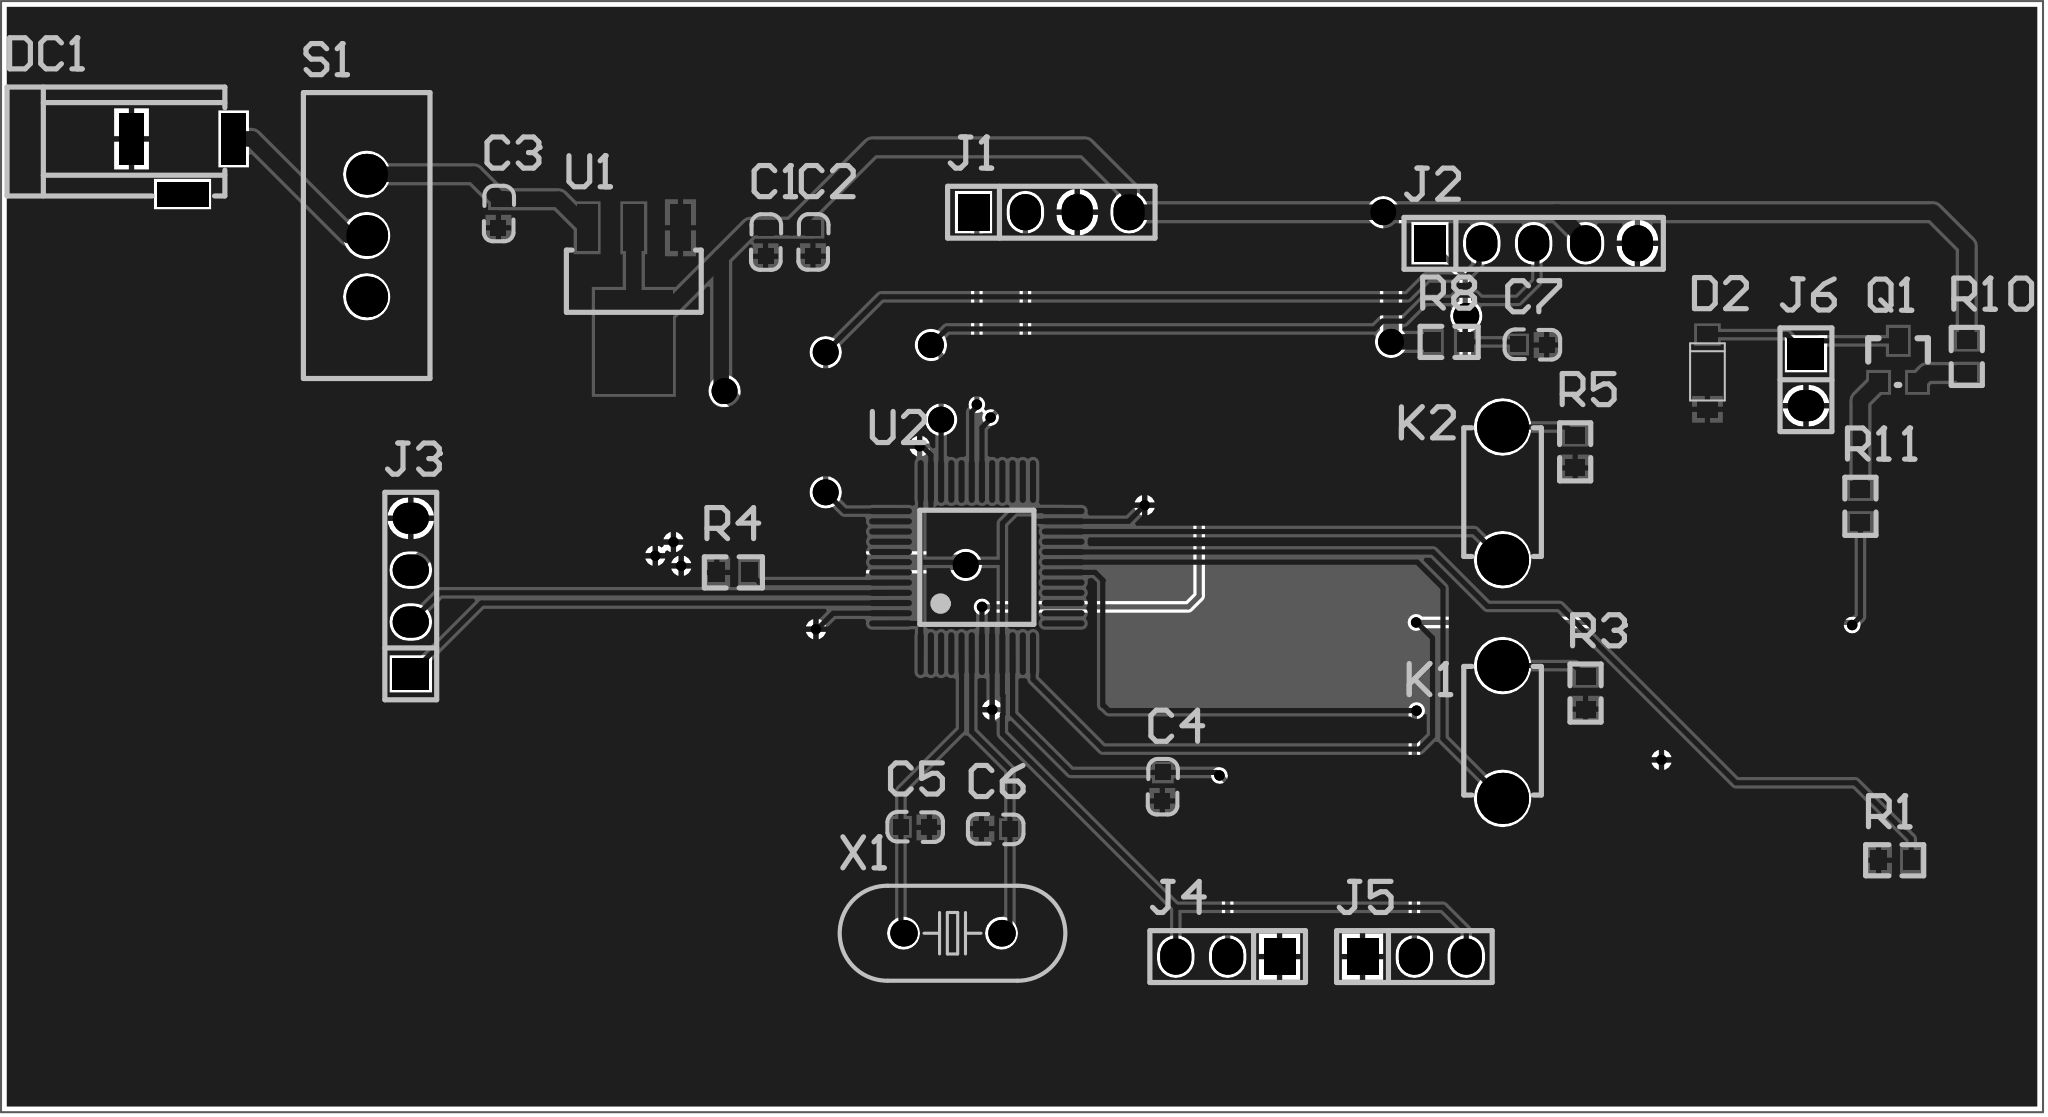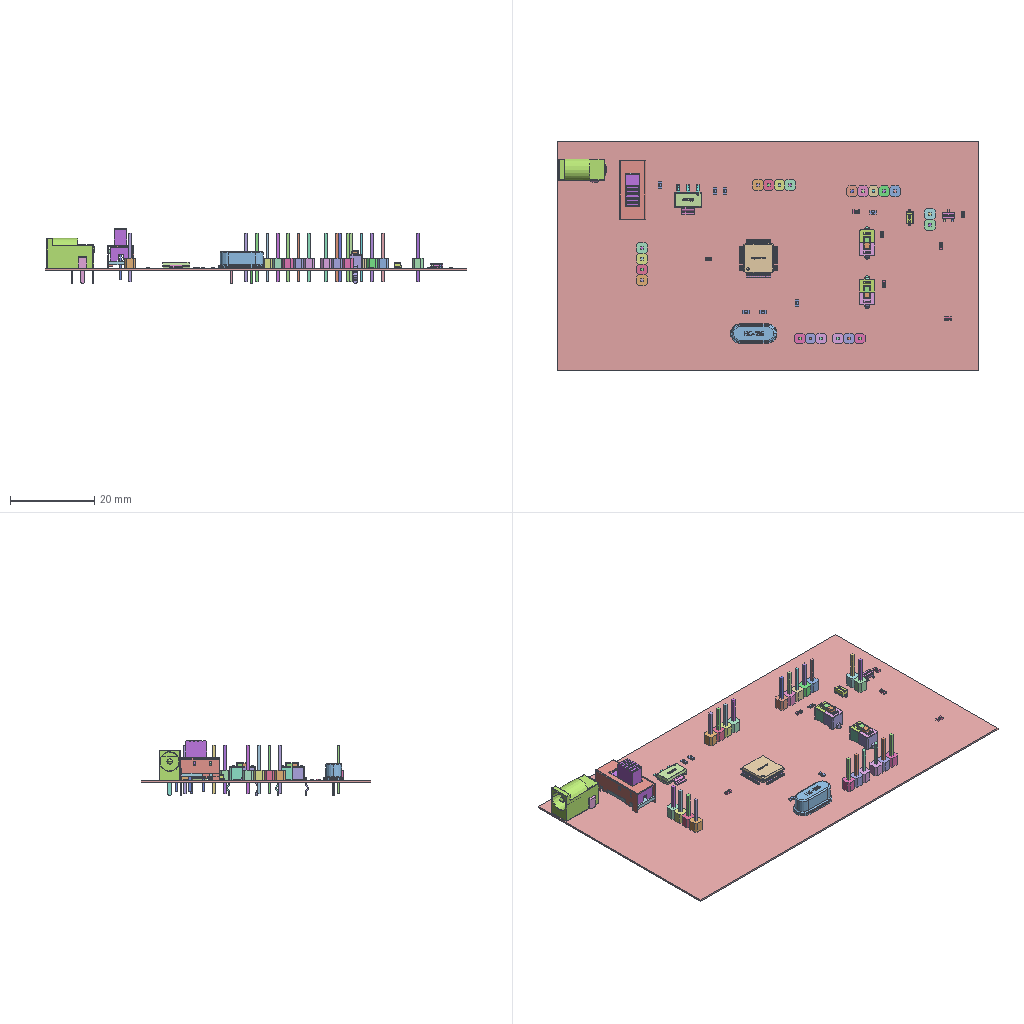Circuit board layout | Altium Designer | box 100 x 54.4 x 13.1 mm
Layer stack:
# Altium Designer layer stack of  (unit mm; dielectric type: 0 none, 1 core, 2 prepreg, 3 surface material)
index,name,kind,layer,copper_thickness_mm,dielectric_type,dielectric_thickness_mm,dielectric_material,dielectric_constant
0,Top Paste,other,,,,,,
1,Top Overlay,other,,,,,,
2,Top Solder,dielectric,,,3,0.0102,Solder Resist,3.5
3,Top Layer,copper,Top Layer,0.0356,,,,
4,Dielectric 1,dielectric,,,0,0.32,FR-4,4.8
5,Bottom Layer,copper,Bottom Layer,0.0356,,,,
6,Bottom Solder,dielectric,,,3,0.0102,Solder Resist,3.5
7,Bottom Overlay,other,,,,,,
8,Bottom Paste,other,,,,,,
# drill layer pairs: low layer,high layer
drill_pair,Top Layer,Bottom Layer
Part placement:
Designator,Comment,Layer,Footprint,Center-X(mm),Center-Y(mm),Rotation
C1,10uF,TopLayer,0603C,37.452,88.201,90
C2,0.1uF,TopLayer,0603C,39.773,88.207,90
C3,10uF,TopLayer,0603C,24.371,89.599,90
C4,0.1uF,TopLayer,0603C,56.883,61.532,90
C5,20pF,TopLayer,0603C,44.767,59.55,180
C6,20pF,TopLayer,0603C,48.71,59.465,0
C7,0.1uF,TopLayer,0603C,74.993,83.172,180
DC1,DC_Socket,TopLayer,DC-002,8.89,91.901,180
J1,Pin HDR1X4,TopLayer,Pin_HDR1X4/2.54mm-S,51.435,89.662,90
J2,Pin HDR1X5,TopLayer,Pin_HDR1X5/2.54mm-S,75.057,88.138,90
J3,Pin HDR1X4,TopLayer,Pin_HDR1X4/2.54mm-S,20.066,70.866,180
K1,KEY,TopLayer,DIP-3X6X4.3,73.533,64.21,90
K2,KEY,TopLayer,DIP-3X6X4.3,73.533,75.894,90
R1,10K,TopLayer,0603R,92.748,57.929,0
R3,10K,TopLayer,0603R,77.597,66.129,90
R4,10K,TopLayer,0603R,35.852,72.025,180
R5,10K,TopLayer,0603R,77.089,77.94,90
R8,10K,TopLayer,0603R,70.904,83.312,180
R10,470,TopLayer,0603R,96.266,82.588,270
R11,470,TopLayer,0603R,91.059,75.273,90
S1,SS-12D10,TopLayer,SS-12D10,17.907,88.519,270
U1,AMS1117,TopLayer,SOT223,30.988,86.106,180
U2,STM32F103C8T6,TopLayer,LQFP48_7X7,47.788,72.262,0
X1,XTAL-2P,TopLayer,OSC_HC-49S,46.596,54.356,360
D2,DIODE,TopLayer,SOD-123,83.566,81.839,90
J4,Pin HDR1X3,TopLayer,Pin_HDR1X3/2.54mm-S,60.071,53.213,270
J5,Pin HDR1X3,TopLayer,Pin_HDR1X3/2.54mm-S,69.215,53.213,90
J6,Pin HDR1X2,TopLayer,Pin_HDR1X2/2.54mm-S,88.392,81.458,0
Q1,PNP,TopLayer,SOT-23,92.9,82.347,0
Pad and via stacks:
# Altium Designer via and pad stacks of  (unit mm). Each distinct definition once, with the count of objects using it.
# via: kind,start_layer,end_layer,hole_mm,diameter_mm,mode(0 simple;1 top-mid-bottom;2 full stack),diameter_per_layer,count,example_net
# pad: kind,layer,hole_mm,hole_type(0 round;1 square;2 slot),plating,top_size,top_shape(1 round;2 rect;3 octagon;9 rounded rect),mid_size,bottom_size,mode,footprint,size_per_layer,count,example
pad,Top Layer,0,0,plated,0.8x0.965,2,0.8x0.965,0.8x0.965,0,0603R,,14,R11.1
pad,Top Layer,0,0,plated,0.762x0.762,2,0.762x0.762,0.762x0.762,0,0603C,,14,C7.1
pad,Top Layer,0,0,plated,0.3x2.1,1,0.3x2.1,0.3x2.1,0,LQFP48 7X7,,48,U2.1
pad,Top Layer,0,0,plated,3.81x5.08,2,3.81x5.08,3.81x5.08,0,SOT223,,1,U1.2
pad,Top Layer,0,0,plated,1.016x2.286,2,1.016x2.286,1.016x2.286,0,SOT223,,3,U1.2
pad,Top Layer,0,0,plated,1x0.8,2,1x0.8,1x0.8,0,SOD-123,,2,D2.K
pad,Top Layer,0,0,plated,0.9144x1.27,2,0.9144x1.27,0.9144x1.27,0,SOT-23,,1,Q1.C
pad,Top Layer,0,0,plated,0.9144x0.9144,2,0.9144x0.9144,0.9144x0.9144,0,SOT-23,,2,Q1.E
pad,Multi-Layer,0.6,0,plated,1.3x1.3,1,1.3x1.3,1.3x1.3,0,OSC HC-49S,,2,X1.2
pad,Multi-Layer,0.8128,0,plated,1.524x1.778,2,1.524x1.778,1.524x1.778,0,Pin HDR1X4/2.54mm-S,,2,J1.1
pad,Multi-Layer,0.8128,0,plated,1.524x1.778,1,1.524x1.778,1.524x1.778,0,Pin HDR1X4/2.54mm-S,,6,J1.2
pad,Multi-Layer,1.2,0,plated,2x2,1,2x2,2x2,0,SS-12D10,,3,S1.1
pad,Multi-Layer,0.6,2,plated,2.5x1.2,2,2.5x1.2,2.5x1.2,0,DC-002,,3,DC1.1
pad,Multi-Layer,1.2,0,plated,2.5x2.5,1,2.5x2.5,2.5x2.5,0,DIP-3X6X4.3,,4,K2.3
pad,Multi-Layer,0.8128,0,plated,1.524x1.778,2,1.524x1.778,1.524x1.778,0,Pin HDR1X2/2.54mm-S,,1,J6.1
pad,Multi-Layer,0.8128,0,plated,1.524x1.778,1,1.524x1.778,1.524x1.778,0,Pin HDR1X2/2.54mm-S,,1,J6.2
pad,Multi-Layer,0.8128,0,plated,1.524x1.778,2,1.524x1.778,1.524x1.778,0,Pin HDR1X3/2.54mm-S,,2,J4.1
pad,Multi-Layer,0.8128,0,plated,1.524x1.778,1,1.524x1.778,1.524x1.778,0,Pin HDR1X3/2.54mm-S,,4,J4.2
pad,Multi-Layer,0.8128,0,plated,1.524x1.778,2,1.524x1.778,1.524x1.778,0,Pin HDR1X5/2.54mm-S,,1,J2.1
pad,Multi-Layer,0.8128,0,plated,1.524x1.778,1,1.524x1.778,1.524x1.778,0,Pin HDR1X5/2.54mm-S,,4,J2.2
via,Top Layer,Bottom Layer,0.254,0.508,0,,15,GND
via,Top Layer,Bottom Layer,0.7112,1.27,0,,9,VCC
Copper pours:
name,layer,net,type(0 solid;1 hatched;2 none)
G,Top Layer,GND,0
G,Bottom Layer,GND,0
Design rules, without the lines most boards share:
# Altium Designer design rules of  (exported by Altium Designer, unit mm)
# columns: name | kind | enabled | priority | scope1 | scope2 | descriptor | typed fields (field=value)
Clearance | 0 | enabled | 1 | All | All | Clearance Constraint (Gap=6mil) (All),(All) | gap=0.1524
PlaneConnect | 6 | enabled | 1 | All | All | Power Plane Connect Rule(Relief Connect )(Expansion=20mil) (Conductor Width=10mil) (Air Gap=10mil) (Entries=4) (All) | relief_conductor_width=0.254 relief_entries=4 relief_expansion=0.508
PolygonConnect | 20 | enabled | 1 | All | All | Polygon Connect Rule(Relief Connect )(Conductor Width=10mil) (Relief Angle=90 Angle) (Entries=4) (Air Gap Width=10mil) (All),(All) | connect_style(0=relief,1=direct,2=none)=0 relief_conductor_width=0.254 relief_entries=4
Width | 2 | enabled | 1 | All | All | Width Constraint (Min=10mil) (Max=50mil) (Preferred=10mil) (All) |
RoutingVias | 11 | enabled | 1 | All | All | Routing Via (MinHoleWidth=10mil) (MaxHoleWidth=10mil) (PreferredHoleWidth=10mil) (MinWidth=20mil) (MaxWidth=50mil) (PreferedWidth=20mil) (All) | via_min_hole=0.254 via_max_hole=0.254 via_preferred_diameter=0.508 via_preferred_hole=0.254
PasteMaskExpansion | 14 | enabled | 1 | All | All | Paste Mask Expansion (Expansion =0mil) (All) | expansion=0
SolderMaskExpansion | 13 | enabled | 1 | All | All | Solder Mask Expansion (Expansion =4mil) (All) | expansion=0.1016
DiffPairsRouting | 51 | enabled | 1 | All | All | Differential Pairs Uncoupled Length using the Gap Constraints (Min=10mil) (Max=10mil) (Prefered=10mil)  and Width Constraints (Min=15mil) (Max=15mil) (Prefered=15mil) (All) |
HoleToHoleClearance | 52 | enabled | 1 | All | All | Hole To Hole Clearance (Gap=10mil) (All),(All) | gap=0.254
MinimumSolderMaskSliver | 53 | enabled | 1 | All | All | Minimum Solder Mask Sliver (Gap=0mil) (All),(All) |
SilkToSolderMaskClearance | 54 | enabled | 1 | IsPad | All | Silk To Solder Mask (Clearance=0mil) (IsPad),(All) |
SilkToSilkClearance | 55 | enabled | 1 | All | All | Silk to Silk (Clearance=0mil) (All),(All) |
Classes set for this board:
# Altium Designer classes of  (member kind: 0 net, 1 component, 2 from-to, 3 pad, 4 layer, 5 differential pair, 6 design channel, 7 polygon, 8 structure, 9 xSignal)
# columns: class name | member kind | superclass | members
Sheet1 | 1 | no | C1; C2; C3; C4; C5; C6; C7; DC1; J1; J2; J3; K1; K2; R1; R3; R4; R5; R8; R10; R11; S1; U1; U2; X1; J4; J5; J6; Q1; D2;